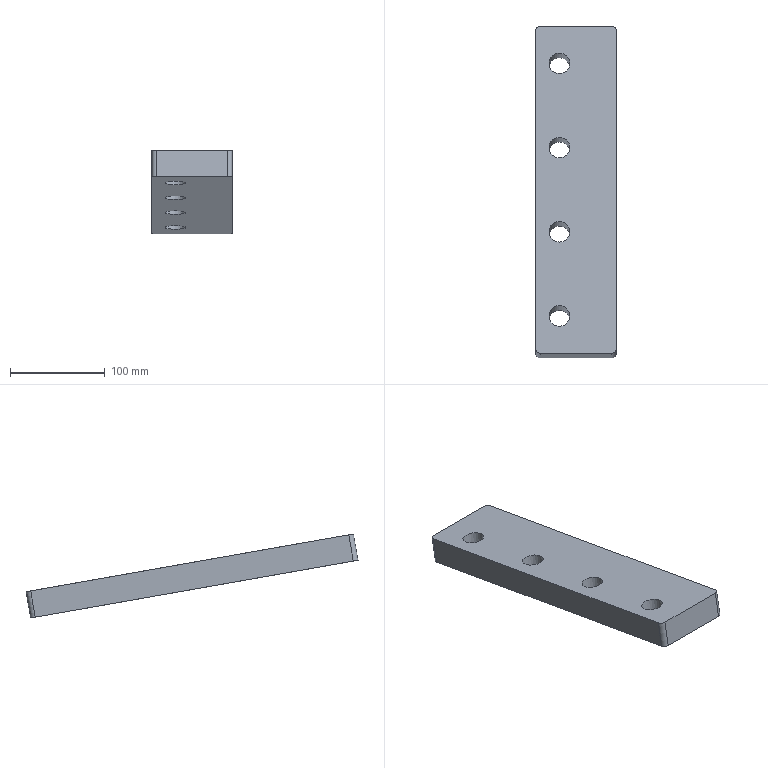Part | NX | features MAIN_BODY 2 | 1 solid | 14 faces | box 85 x 349.545 x 88.351 mm | volume 789824 mm3 | cylinder 8 | plane 6 | commonest cylinder face diameters 10 x4 22 x4
STEP:
#1=CARTESIAN_POINT('',(-1343.,-839.967,-165.111));
#2=VERTEX_POINT('',#1);
#3=CARTESIAN_POINT('',(-1343.,-1174.802,-106.071));
#4=VERTEX_POINT('',#3);
#5=CARTESIAN_POINT('',(-1343.,-982.764,-139.932));
#6=DIRECTION('',(0.,-0.9848,0.1736));
#7=VECTOR('',#6,1000.);
#8=LINE('',#5,#7);
#9=EDGE_CURVE('',#2,#4,#8,.T.);
#10=ORIENTED_EDGE('',*,*,#9,.F.);
#11=CARTESIAN_POINT('',(-1348.,-835.043,-165.979));
#12=VERTEX_POINT('',#11);
#13=CARTESIAN_POINT('',(-1348.,-839.967,-165.111));
#14=DIRECTION('',(0.,-0.1736,-0.9848));
#15=DIRECTION('',(0.,0.9848,-0.1736));
#16=AXIS2_PLACEMENT_3D('',#13,#14,#15);
#17=CIRCLE('',#16,5.);
#18=EDGE_CURVE('',#2,#12,#17,.F.);
#19=ORIENTED_EDGE('',*,*,#18,.T.);
#20=CARTESIAN_POINT('',(-1423.,-835.043,-165.979));
#21=VERTEX_POINT('',#20);
#22=CARTESIAN_POINT('',(-1428.,-835.043,-165.979));
#23=DIRECTION('',(1.,0.,0.));
#24=VECTOR('',#23,1000.);
#25=LINE('',#22,#24);
#26=EDGE_CURVE('',#21,#12,#25,.T.);
#27=ORIENTED_EDGE('',*,*,#26,.F.);
#28=CARTESIAN_POINT('',(-1428.,-839.967,-165.111));
#29=VERTEX_POINT('',#28);
#30=CARTESIAN_POINT('',(-1423.,-839.967,-165.111));
#31=DIRECTION('',(0.,-0.1736,-0.9848));
#32=DIRECTION('',(0.,0.9848,-0.1736));
#33=AXIS2_PLACEMENT_3D('',#30,#31,#32);
#34=CIRCLE('',#33,5.);
#35=EDGE_CURVE('',#21,#29,#34,.F.);
#36=ORIENTED_EDGE('',*,*,#35,.T.);
#37=CARTESIAN_POINT('',(-1428.,-1174.802,-106.071));
#38=VERTEX_POINT('',#37);
#39=CARTESIAN_POINT('',(-1428.,-1179.726,-105.203));
#40=DIRECTION('',(0.,0.9848,-0.1736));
#41=VECTOR('',#40,1000.);
#42=LINE('',#39,#41);
#43=EDGE_CURVE('',#38,#29,#42,.T.);
#44=ORIENTED_EDGE('',*,*,#43,.F.);
#45=CARTESIAN_POINT('',(-1423.,-1179.726,-105.203));
#46=VERTEX_POINT('',#45);
#47=CARTESIAN_POINT('',(-1423.,-1174.802,-106.071));
#48=DIRECTION('',(0.,-0.1736,-0.9848));
#49=DIRECTION('',(0.,0.9848,-0.1736));
#50=AXIS2_PLACEMENT_3D('',#47,#48,#49);
#51=CIRCLE('',#50,5.);
#52=EDGE_CURVE('',#38,#46,#51,.F.);
#53=ORIENTED_EDGE('',*,*,#52,.T.);
#54=CARTESIAN_POINT('',(-1348.,-1179.726,-105.203));
#55=VERTEX_POINT('',#54);
#56=CARTESIAN_POINT('',(-1343.,-1179.726,-105.203));
#57=DIRECTION('',(-1.,0.,0.));
#58=VECTOR('',#57,1000.);
#59=LINE('',#56,#58);
#60=EDGE_CURVE('',#55,#46,#59,.T.);
#61=ORIENTED_EDGE('',*,*,#60,.F.);
#62=CARTESIAN_POINT('',(-1348.,-1174.802,-106.071));
#63=DIRECTION('',(0.,-0.1736,-0.9848));
#64=DIRECTION('',(0.,0.9848,-0.1736));
#65=AXIS2_PLACEMENT_3D('',#62,#63,#64);
#66=CIRCLE('',#65,5.);
#67=EDGE_CURVE('',#55,#4,#66,.F.);
#68=ORIENTED_EDGE('',*,*,#67,.T.);
#69=EDGE_LOOP('',(#10,#19,#27,#36,#44,#53,#61,#68));
#70=FACE_BOUND('',#69,.T.);
#71=CARTESIAN_POINT('',(-1403.,-1129.501,-114.059));
#72=VERTEX_POINT('',#71);
#73=CARTESIAN_POINT('',(-1403.,-1140.334,-112.148));
#74=DIRECTION('',(0.,-0.1736,-0.9848));
#75=DIRECTION('',(0.,0.9848,-0.1736));
#76=AXIS2_PLACEMENT_3D('',#73,#74,#75);
#77=CIRCLE('',#76,11.);
#78=EDGE_CURVE('',#72,#72,#77,.T.);
#79=ORIENTED_EDGE('',*,*,#78,.T.);
#80=EDGE_LOOP('',(#79));
#81=FACE_BOUND('',#80,.T.);
#82=CARTESIAN_POINT('',(-1403.,-863.603,-160.944));
#83=VERTEX_POINT('',#82);
#84=CARTESIAN_POINT('',(-1403.,-874.436,-159.033));
#85=DIRECTION('',(0.,-0.1736,-0.9848));
#86=DIRECTION('',(0.,0.9848,-0.1736));
#87=AXIS2_PLACEMENT_3D('',#84,#85,#86);
#88=CIRCLE('',#87,11.);
#89=EDGE_CURVE('',#83,#83,#88,.T.);
#90=ORIENTED_EDGE('',*,*,#89,.T.);
#91=EDGE_LOOP('',(#90));
#92=FACE_BOUND('',#91,.T.);
#93=CARTESIAN_POINT('',(-1403.,-952.235,-145.315));
#94=VERTEX_POINT('',#93);
#95=CARTESIAN_POINT('',(-1403.,-963.068,-143.405));
#96=DIRECTION('',(0.,-0.1736,-0.9848));
#97=DIRECTION('',(0.,0.9848,-0.1736));
#98=AXIS2_PLACEMENT_3D('',#95,#96,#97);
#99=CIRCLE('',#98,11.);
#100=EDGE_CURVE('',#94,#94,#99,.T.);
#101=ORIENTED_EDGE('',*,*,#100,.T.);
#102=EDGE_LOOP('',(#101));
#103=FACE_BOUND('',#102,.T.);
#104=CARTESIAN_POINT('',(-1403.,-1040.868,-129.687));
#105=VERTEX_POINT('',#104);
#106=CARTESIAN_POINT('',(-1403.,-1051.701,-127.777));
#107=DIRECTION('',(0.,-0.1736,-0.9848));
#108=DIRECTION('',(0.,0.9848,-0.1736));
#109=AXIS2_PLACEMENT_3D('',#106,#107,#108);
#110=CIRCLE('',#109,11.);
#111=EDGE_CURVE('',#105,#105,#110,.F.);
#112=ORIENTED_EDGE('',*,*,#111,.F.);
#113=EDGE_LOOP('',(#112));
#114=FACE_BOUND('',#113,.T.);
#115=CARTESIAN_POINT('',(-1428.,-1179.726,-105.203));
#116=DIRECTION('',(0.,-0.1736,-0.9848));
#117=DIRECTION('',(0.,0.9848,-0.1736));
#118=AXIS2_PLACEMENT_3D('',#115,#116,#117);
#119=PLANE('',#118);
#120=ADVANCED_FACE('',(#70,#81,#92,#103,#114),#119,.F.);
#121=CARTESIAN_POINT('',(-1423.,-839.905,-193.554));
#122=VERTEX_POINT('',#121);
#123=CARTESIAN_POINT('',(-1348.,-839.905,-193.554));
#124=VERTEX_POINT('',#123);
#125=CARTESIAN_POINT('',(-1428.,-839.905,-193.554));
#126=DIRECTION('',(1.,0.,0.));
#127=VECTOR('',#126,1000.);
#128=LINE('',#125,#127);
#129=EDGE_CURVE('',#122,#124,#128,.T.);
#130=ORIENTED_EDGE('',*,*,#129,.T.);
#131=CARTESIAN_POINT('',(-1343.,-844.829,-192.686));
#132=VERTEX_POINT('',#131);
#133=CARTESIAN_POINT('',(-1348.,-844.829,-192.686));
#134=DIRECTION('',(0.,-0.1736,-0.9848));
#135=DIRECTION('',(0.,0.9848,-0.1736));
#136=AXIS2_PLACEMENT_3D('',#133,#134,#135);
#137=CIRCLE('',#136,5.);
#138=EDGE_CURVE('',#124,#132,#137,.T.);
#139=ORIENTED_EDGE('',*,*,#138,.T.);
#140=CARTESIAN_POINT('',(-1343.,-1179.664,-133.645));
#141=VERTEX_POINT('',#140);
#142=CARTESIAN_POINT('',(-1343.,-987.627,-167.507));
#143=DIRECTION('',(0.,-0.9848,0.1736));
#144=VECTOR('',#143,1000.);
#145=LINE('',#142,#144);
#146=EDGE_CURVE('',#132,#141,#145,.T.);
#147=ORIENTED_EDGE('',*,*,#146,.T.);
#148=CARTESIAN_POINT('',(-1348.,-1184.588,-132.777));
#149=VERTEX_POINT('',#148);
#150=CARTESIAN_POINT('',(-1348.,-1179.664,-133.645));
#151=DIRECTION('',(0.,-0.1736,-0.9848));
#152=DIRECTION('',(0.,0.9848,-0.1736));
#153=AXIS2_PLACEMENT_3D('',#150,#151,#152);
#154=CIRCLE('',#153,5.);
#155=EDGE_CURVE('',#141,#149,#154,.T.);
#156=ORIENTED_EDGE('',*,*,#155,.T.);
#157=CARTESIAN_POINT('',(-1423.,-1184.588,-132.777));
#158=VERTEX_POINT('',#157);
#159=CARTESIAN_POINT('',(-1343.,-1184.588,-132.777));
#160=DIRECTION('',(-1.,0.,0.));
#161=VECTOR('',#160,1000.);
#162=LINE('',#159,#161);
#163=EDGE_CURVE('',#149,#158,#162,.T.);
#164=ORIENTED_EDGE('',*,*,#163,.T.);
#165=CARTESIAN_POINT('',(-1428.,-1179.664,-133.645));
#166=VERTEX_POINT('',#165);
#167=CARTESIAN_POINT('',(-1423.,-1179.664,-133.645));
#168=DIRECTION('',(0.,-0.1736,-0.9848));
#169=DIRECTION('',(0.,0.9848,-0.1736));
#170=AXIS2_PLACEMENT_3D('',#167,#168,#169);
#171=CIRCLE('',#170,5.);
#172=EDGE_CURVE('',#158,#166,#171,.T.);
#173=ORIENTED_EDGE('',*,*,#172,.T.);
#174=CARTESIAN_POINT('',(-1428.,-844.829,-192.686));
#175=VERTEX_POINT('',#174);
#176=CARTESIAN_POINT('',(-1428.,-1184.588,-132.777));
#177=DIRECTION('',(0.,0.9848,-0.1736));
#178=VECTOR('',#177,1000.);
#179=LINE('',#176,#178);
#180=EDGE_CURVE('',#166,#175,#179,.T.);
#181=ORIENTED_EDGE('',*,*,#180,.T.);
#182=CARTESIAN_POINT('',(-1423.,-844.829,-192.686));
#183=DIRECTION('',(0.,-0.1736,-0.9848));
#184=DIRECTION('',(0.,0.9848,-0.1736));
#185=AXIS2_PLACEMENT_3D('',#182,#183,#184);
#186=CIRCLE('',#185,5.);
#187=EDGE_CURVE('',#175,#122,#186,.T.);
#188=ORIENTED_EDGE('',*,*,#187,.T.);
#189=EDGE_LOOP('',(#130,#139,#147,#156,#164,#173,#181,#188));
#190=FACE_BOUND('',#189,.T.);
#191=CARTESIAN_POINT('',(-1403.,-1134.363,-141.633));
#192=VERTEX_POINT('',#191);
#193=CARTESIAN_POINT('',(-1403.,-1145.196,-139.723));
#194=DIRECTION('',(0.,-0.1736,-0.9848));
#195=DIRECTION('',(0.,0.9848,-0.1736));
#196=AXIS2_PLACEMENT_3D('',#193,#194,#195);
#197=CIRCLE('',#196,11.);
#198=EDGE_CURVE('',#192,#192,#197,.T.);
#199=ORIENTED_EDGE('',*,*,#198,.F.);
#200=EDGE_LOOP('',(#199));
#201=FACE_BOUND('',#200,.T.);
#202=CARTESIAN_POINT('',(-1403.,-868.465,-188.518));
#203=VERTEX_POINT('',#202);
#204=CARTESIAN_POINT('',(-1403.,-879.298,-186.608));
#205=DIRECTION('',(0.,-0.1736,-0.9848));
#206=DIRECTION('',(0.,0.9848,-0.1736));
#207=AXIS2_PLACEMENT_3D('',#204,#205,#206);
#208=CIRCLE('',#207,11.);
#209=EDGE_CURVE('',#203,#203,#208,.T.);
#210=ORIENTED_EDGE('',*,*,#209,.F.);
#211=EDGE_LOOP('',(#210));
#212=FACE_BOUND('',#211,.T.);
#213=CARTESIAN_POINT('',(-1403.,-957.098,-172.89));
#214=VERTEX_POINT('',#213);
#215=CARTESIAN_POINT('',(-1403.,-967.93,-170.98));
#216=DIRECTION('',(0.,-0.1736,-0.9848));
#217=DIRECTION('',(0.,0.9848,-0.1736));
#218=AXIS2_PLACEMENT_3D('',#215,#216,#217);
#219=CIRCLE('',#218,11.);
#220=EDGE_CURVE('',#214,#214,#219,.T.);
#221=ORIENTED_EDGE('',*,*,#220,.F.);
#222=EDGE_LOOP('',(#221));
#223=FACE_BOUND('',#222,.T.);
#224=CARTESIAN_POINT('',(-1403.,-1045.73,-157.262));
#225=VERTEX_POINT('',#224);
#226=CARTESIAN_POINT('',(-1403.,-1056.563,-155.351));
#227=DIRECTION('',(0.,-0.1736,-0.9848));
#228=DIRECTION('',(0.,0.9848,-0.1736));
#229=AXIS2_PLACEMENT_3D('',#226,#227,#228);
#230=CIRCLE('',#229,11.);
#231=EDGE_CURVE('',#225,#225,#230,.F.);
#232=ORIENTED_EDGE('',*,*,#231,.T.);
#233=EDGE_LOOP('',(#232));
#234=FACE_BOUND('',#233,.T.);
#235=CARTESIAN_POINT('',(-1428.,-1184.588,-132.777));
#236=DIRECTION('',(0.,-0.1736,-0.9848));
#237=DIRECTION('',(0.,0.9848,-0.1736));
#238=AXIS2_PLACEMENT_3D('',#235,#236,#237);
#239=PLANE('',#238);
#240=ADVANCED_FACE('',(#190,#201,#212,#223,#234),#239,.T.);
#241=ORIENTED_EDGE('',*,*,#163,.F.);
#242=CARTESIAN_POINT('',(-1348.,-1179.726,-105.203));
#243=DIRECTION('',(0.,-0.1736,-0.9848));
#244=VECTOR('',#243,1000.);
#245=LINE('',#242,#244);
#246=EDGE_CURVE('',#149,#55,#245,.F.);
#247=ORIENTED_EDGE('',*,*,#246,.T.);
#248=ORIENTED_EDGE('',*,*,#60,.T.);
#249=CARTESIAN_POINT('',(-1423.,-1179.726,-105.203));
#250=DIRECTION('',(0.,-0.1736,-0.9848));
#251=VECTOR('',#250,1000.);
#252=LINE('',#249,#251);
#253=EDGE_CURVE('',#46,#158,#252,.T.);
#254=ORIENTED_EDGE('',*,*,#253,.T.);
#255=EDGE_LOOP('',(#241,#247,#248,#254));
#256=FACE_BOUND('',#255,.T.);
#257=CARTESIAN_POINT('',(-1343.,-1179.726,-105.203));
#258=DIRECTION('',(0.,-0.9848,0.1736));
#259=DIRECTION('',(1.,0.,0.));
#260=AXIS2_PLACEMENT_3D('',#257,#258,#259);
#261=PLANE('',#260);
#262=ADVANCED_FACE('',(#256),#261,.T.);
#263=ORIENTED_EDGE('',*,*,#43,.T.);
#264=CARTESIAN_POINT('',(-1428.,-839.967,-165.111));
#265=DIRECTION('',(0.,-0.1736,-0.9848));
#266=VECTOR('',#265,1000.);
#267=LINE('',#264,#266);
#268=EDGE_CURVE('',#29,#175,#267,.T.);
#269=ORIENTED_EDGE('',*,*,#268,.T.);
#270=ORIENTED_EDGE('',*,*,#180,.F.);
#271=CARTESIAN_POINT('',(-1428.,-1174.802,-106.071));
#272=DIRECTION('',(0.,-0.1736,-0.9848));
#273=VECTOR('',#272,1000.);
#274=LINE('',#271,#273);
#275=EDGE_CURVE('',#166,#38,#274,.F.);
#276=ORIENTED_EDGE('',*,*,#275,.T.);
#277=EDGE_LOOP('',(#263,#269,#270,#276));
#278=FACE_BOUND('',#277,.T.);
#279=CARTESIAN_POINT('',(-1428.,-1179.726,-105.203));
#280=DIRECTION('',(-1.,0.,0.));
#281=DIRECTION('',(0.,-0.9848,0.1736));
#282=AXIS2_PLACEMENT_3D('',#279,#280,#281);
#283=PLANE('',#282);
#284=ADVANCED_FACE('',(#278),#283,.T.);
#285=ORIENTED_EDGE('',*,*,#26,.T.);
#286=CARTESIAN_POINT('',(-1348.,-835.043,-165.979));
#287=DIRECTION('',(0.,-0.1736,-0.9848));
#288=VECTOR('',#287,1000.);
#289=LINE('',#286,#288);
#290=EDGE_CURVE('',#12,#124,#289,.T.);
#291=ORIENTED_EDGE('',*,*,#290,.T.);
#292=ORIENTED_EDGE('',*,*,#129,.F.);
#293=CARTESIAN_POINT('',(-1423.,-835.043,-165.979));
#294=DIRECTION('',(0.,-0.1736,-0.9848));
#295=VECTOR('',#294,1000.);
#296=LINE('',#293,#295);
#297=EDGE_CURVE('',#122,#21,#296,.F.);
#298=ORIENTED_EDGE('',*,*,#297,.T.);
#299=EDGE_LOOP('',(#285,#291,#292,#298));
#300=FACE_BOUND('',#299,.T.);
#301=CARTESIAN_POINT('',(-1428.,-835.043,-165.979));
#302=DIRECTION('',(0.,0.9848,-0.1736));
#303=DIRECTION('',(0.,0.1736,0.9848));
#304=AXIS2_PLACEMENT_3D('',#301,#302,#303);
#305=PLANE('',#304);
#306=ADVANCED_FACE('',(#300),#305,.T.);
#307=ORIENTED_EDGE('',*,*,#146,.F.);
#308=CARTESIAN_POINT('',(-1343.,-839.967,-165.111));
#309=DIRECTION('',(0.,-0.1736,-0.9848));
#310=VECTOR('',#309,1000.);
#311=LINE('',#308,#310);
#312=EDGE_CURVE('',#132,#2,#311,.F.);
#313=ORIENTED_EDGE('',*,*,#312,.T.);
#314=ORIENTED_EDGE('',*,*,#9,.T.);
#315=CARTESIAN_POINT('',(-1343.,-1174.802,-106.071));
#316=DIRECTION('',(0.,-0.1736,-0.9848));
#317=VECTOR('',#316,1000.);
#318=LINE('',#315,#317);
#319=EDGE_CURVE('',#4,#141,#318,.T.);
#320=ORIENTED_EDGE('',*,*,#319,.T.);
#321=EDGE_LOOP('',(#307,#313,#314,#320));
#322=FACE_BOUND('',#321,.T.);
#323=CARTESIAN_POINT('',(-1343.,-982.764,-139.932));
#324=DIRECTION('',(1.,0.,0.));
#325=DIRECTION('',(0.,0.1736,0.9848));
#326=AXIS2_PLACEMENT_3D('',#323,#324,#325);
#327=PLANE('',#326);
#328=ADVANCED_FACE('',(#322),#327,.T.);
#329=ORIENTED_EDGE('',*,*,#198,.T.);
#330=EDGE_LOOP('',(#329));
#331=FACE_BOUND('',#330,.T.);
#332=ORIENTED_EDGE('',*,*,#78,.F.);
#333=EDGE_LOOP('',(#332));
#334=FACE_BOUND('',#333,.T.);
#335=CARTESIAN_POINT('',(-1403.,-1140.334,-112.148));
#336=DIRECTION('',(0.,-0.1736,-0.9848));
#337=DIRECTION('',(0.,0.9848,-0.1736));
#338=AXIS2_PLACEMENT_3D('',#335,#336,#337);
#339=CYLINDRICAL_SURFACE('',#338,11.);
#340=ADVANCED_FACE('',(#331,#334),#339,.F.);
#341=ORIENTED_EDGE('',*,*,#209,.T.);
#342=EDGE_LOOP('',(#341));
#343=FACE_BOUND('',#342,.T.);
#344=ORIENTED_EDGE('',*,*,#89,.F.);
#345=EDGE_LOOP('',(#344));
#346=FACE_BOUND('',#345,.T.);
#347=CARTESIAN_POINT('',(-1403.,-874.436,-159.033));
#348=DIRECTION('',(0.,-0.1736,-0.9848));
#349=DIRECTION('',(0.,0.9848,-0.1736));
#350=AXIS2_PLACEMENT_3D('',#347,#348,#349);
#351=CYLINDRICAL_SURFACE('',#350,11.);
#352=ADVANCED_FACE('',(#343,#346),#351,.F.);
#353=ORIENTED_EDGE('',*,*,#18,.F.);
#354=ORIENTED_EDGE('',*,*,#312,.F.);
#355=ORIENTED_EDGE('',*,*,#138,.F.);
#356=ORIENTED_EDGE('',*,*,#290,.F.);
#357=EDGE_LOOP('',(#353,#354,#355,#356));
#358=FACE_BOUND('',#357,.T.);
#359=CARTESIAN_POINT('',(-1348.,-839.967,-165.111));
#360=DIRECTION('',(0.,-0.1736,-0.9848));
#361=DIRECTION('',(0.,0.9848,-0.1736));
#362=AXIS2_PLACEMENT_3D('',#359,#360,#361);
#363=CYLINDRICAL_SURFACE('',#362,5.);
#364=ADVANCED_FACE('',(#358),#363,.T.);
#365=ORIENTED_EDGE('',*,*,#35,.F.);
#366=ORIENTED_EDGE('',*,*,#297,.F.);
#367=ORIENTED_EDGE('',*,*,#187,.F.);
#368=ORIENTED_EDGE('',*,*,#268,.F.);
#369=EDGE_LOOP('',(#365,#366,#367,#368));
#370=FACE_BOUND('',#369,.T.);
#371=CARTESIAN_POINT('',(-1423.,-839.967,-165.111));
#372=DIRECTION('',(0.,-0.1736,-0.9848));
#373=DIRECTION('',(0.,0.9848,-0.1736));
#374=AXIS2_PLACEMENT_3D('',#371,#372,#373);
#375=CYLINDRICAL_SURFACE('',#374,5.);
#376=ADVANCED_FACE('',(#370),#375,.T.);
#377=ORIENTED_EDGE('',*,*,#67,.F.);
#378=ORIENTED_EDGE('',*,*,#246,.F.);
#379=ORIENTED_EDGE('',*,*,#155,.F.);
#380=ORIENTED_EDGE('',*,*,#319,.F.);
#381=EDGE_LOOP('',(#377,#378,#379,#380));
#382=FACE_BOUND('',#381,.T.);
#383=CARTESIAN_POINT('',(-1348.,-1174.802,-106.071));
#384=DIRECTION('',(0.,-0.1736,-0.9848));
#385=DIRECTION('',(0.,0.9848,-0.1736));
#386=AXIS2_PLACEMENT_3D('',#383,#384,#385);
#387=CYLINDRICAL_SURFACE('',#386,5.);
#388=ADVANCED_FACE('',(#382),#387,.T.);
#389=ORIENTED_EDGE('',*,*,#52,.F.);
#390=ORIENTED_EDGE('',*,*,#275,.F.);
#391=ORIENTED_EDGE('',*,*,#172,.F.);
#392=ORIENTED_EDGE('',*,*,#253,.F.);
#393=EDGE_LOOP('',(#389,#390,#391,#392));
#394=FACE_BOUND('',#393,.T.);
#395=CARTESIAN_POINT('',(-1423.,-1174.802,-106.071));
#396=DIRECTION('',(0.,-0.1736,-0.9848));
#397=DIRECTION('',(0.,0.9848,-0.1736));
#398=AXIS2_PLACEMENT_3D('',#395,#396,#397);
#399=CYLINDRICAL_SURFACE('',#398,5.);
#400=ADVANCED_FACE('',(#394),#399,.T.);
#401=ORIENTED_EDGE('',*,*,#220,.T.);
#402=EDGE_LOOP('',(#401));
#403=FACE_BOUND('',#402,.T.);
#404=ORIENTED_EDGE('',*,*,#100,.F.);
#405=EDGE_LOOP('',(#404));
#406=FACE_BOUND('',#405,.T.);
#407=CARTESIAN_POINT('',(-1403.,-980.433,-241.886));
#408=DIRECTION('',(0.,0.1736,0.9848));
#409=DIRECTION('',(0.,-0.9848,0.1736));
#410=AXIS2_PLACEMENT_3D('',#407,#408,#409);
#411=CYLINDRICAL_SURFACE('',#410,11.);
#412=ADVANCED_FACE('',(#403,#406),#411,.F.);
#413=ORIENTED_EDGE('',*,*,#231,.F.);
#414=EDGE_LOOP('',(#413));
#415=FACE_BOUND('',#414,.T.);
#416=ORIENTED_EDGE('',*,*,#111,.T.);
#417=EDGE_LOOP('',(#416));
#418=FACE_BOUND('',#417,.T.);
#419=CARTESIAN_POINT('',(-1403.,-1034.336,-29.296));
#420=DIRECTION('',(0.,-0.1736,-0.9848));
#421=DIRECTION('',(0.,0.9848,-0.1736));
#422=AXIS2_PLACEMENT_3D('',#419,#420,#421);
#423=CYLINDRICAL_SURFACE('',#422,11.);
#424=ADVANCED_FACE('',(#415,#418),#423,.F.);
#425=CLOSED_SHELL('',(#120,#240,#262,#284,#306,#328,#340,#352,#364,#376,#388,#400,#412,#424));
#426=MANIFOLD_SOLID_BREP('',#425);
#427=(LENGTH_UNIT()NAMED_UNIT(*)SI_UNIT(.MILLI.,.METRE.));
#428=UNCERTAINTY_MEASURE_WITH_UNIT(LENGTH_MEASURE(0.00001),#427,'','');
#429=(NAMED_UNIT(*)PLANE_ANGLE_UNIT()SI_UNIT($,.RADIAN.));
#430=(NAMED_UNIT(*)SI_UNIT($,.STERADIAN.)SOLID_ANGLE_UNIT());
#431=(GEOMETRIC_REPRESENTATION_CONTEXT(3)GLOBAL_UNCERTAINTY_ASSIGNED_CONTEXT((#428))GLOBAL_UNIT_ASSIGNED_CONTEXT((#427,#429,#430))REPRESENTATION_CONTEXT('',''));
#432=ADVANCED_BREP_SHAPE_REPRESENTATION('',(#426),#431);